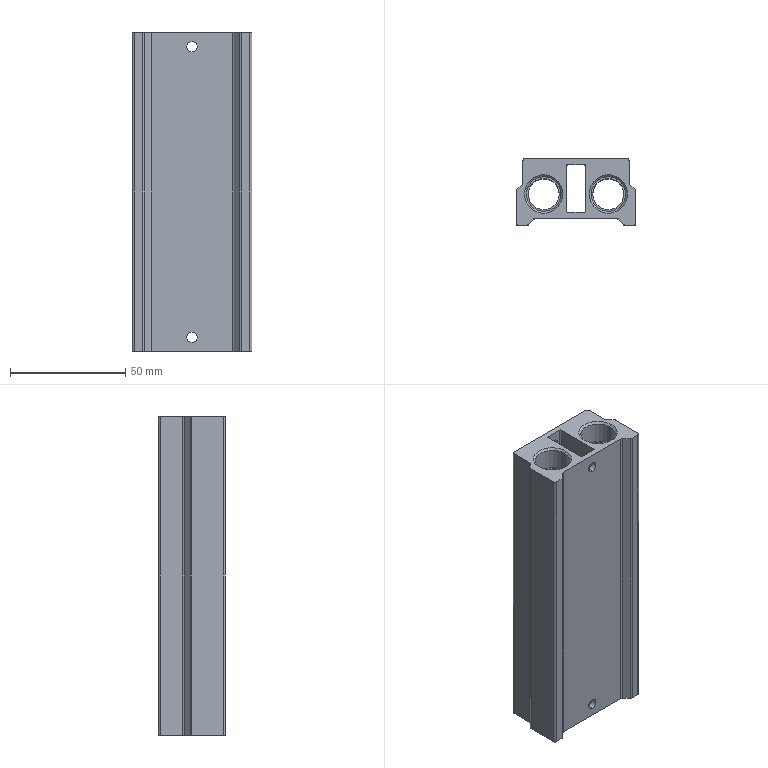Part | SolidWorks | features BaseBody 1 | 1 solid | 130 faces | box 52 x 29 x 138 mm | volume 103703 mm3 | cylinder 68 | plane 38 | cone 24 | commonest cylinder face diameters 3.242 x16 14 x16 2 x12 4.5 x8 14.95 x8 1 x4